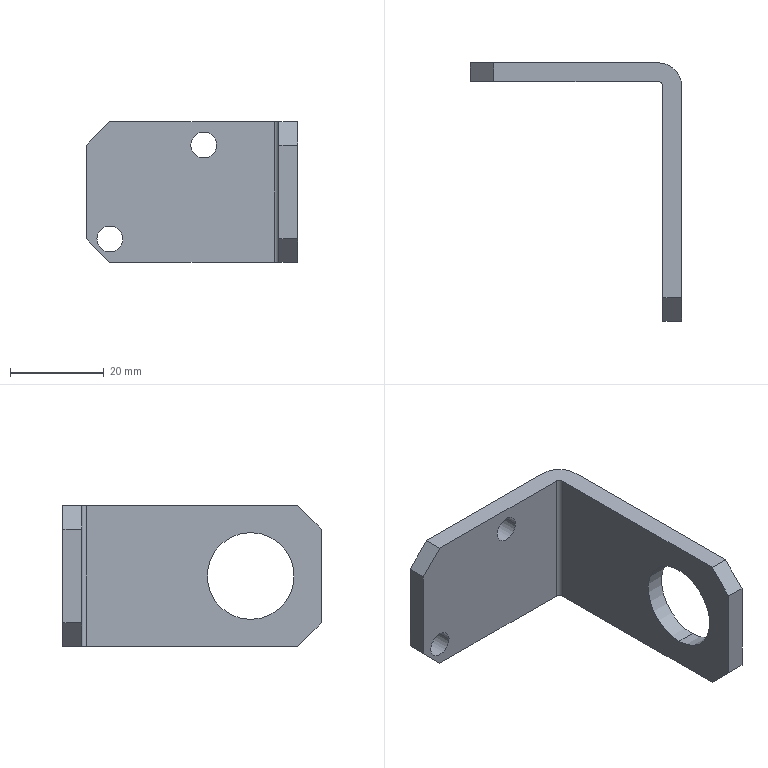Part | SolidWorks | features ICE 2, Chamfer 1, Extrusion 1 | 1 solid | 20 faces | box 45 x 55 x 30 mm | volume 9900 mm3 | plane 12 | cylinder 8 | commonest cylinder face diameters 5.5 x4 18.5 x2 2 x1 10 x1
STEP:
#1=CARTESIAN_POINT('',(7.75,-4.,5.));
#2=VERTEX_POINT('',#1);
#3=CARTESIAN_POINT('',(2.25,-4.,5.));
#4=VERTEX_POINT('',#3);
#5=CARTESIAN_POINT('',(5.,-4.,5.));
#6=DIRECTION('',(0.,1.,0.));
#7=DIRECTION('',(0.,0.,1.));
#8=AXIS2_PLACEMENT_3D('',#5,#6,#7);
#9=CIRCLE('',#8,2.75);
#10=EDGE_CURVE('',#2,#4,#9,.T.);
#11=ORIENTED_EDGE('',*,*,#10,.F.);
#12=CARTESIAN_POINT('',(7.75,0.,5.));
#13=VERTEX_POINT('',#12);
#14=CARTESIAN_POINT('',(7.75,-30.,5.));
#15=DIRECTION('',(0.,1.,0.));
#16=VECTOR('',#15,1000.);
#17=LINE('',#14,#16);
#18=EDGE_CURVE('',#2,#13,#17,.T.);
#19=ORIENTED_EDGE('',*,*,#18,.T.);
#20=CARTESIAN_POINT('',(2.25,0.,5.));
#21=VERTEX_POINT('',#20);
#22=CARTESIAN_POINT('',(5.,0.,5.));
#23=DIRECTION('',(0.,1.,0.));
#24=DIRECTION('',(-1.,0.,0.));
#25=AXIS2_PLACEMENT_3D('',#22,#23,#24);
#26=CIRCLE('',#25,2.75);
#27=EDGE_CURVE('',#13,#21,#26,.T.);
#28=ORIENTED_EDGE('',*,*,#27,.T.);
#29=CARTESIAN_POINT('',(2.25,-30.,5.));
#30=DIRECTION('',(0.,1.,0.));
#31=VECTOR('',#30,1000.);
#32=LINE('',#29,#31);
#33=EDGE_CURVE('',#4,#21,#32,.T.);
#34=ORIENTED_EDGE('',*,*,#33,.F.);
#35=EDGE_LOOP('',(#11,#19,#28,#34));
#36=FACE_OUTER_BOUND('',#35,.T.);
#37=CARTESIAN_POINT('',(5.,-30.,5.));
#38=DIRECTION('',(0.,1.,0.));
#39=DIRECTION('',(-1.,0.,0.));
#40=AXIS2_PLACEMENT_3D('',#37,#38,#39);
#41=CYLINDRICAL_SURFACE('',#40,2.75);
#42=ADVANCED_FACE('',(#36),#41,.F.);
#43=CARTESIAN_POINT('',(27.75,-4.,25.));
#44=VERTEX_POINT('',#43);
#45=CARTESIAN_POINT('',(22.25,-4.,25.));
#46=VERTEX_POINT('',#45);
#47=CARTESIAN_POINT('',(25.,-4.,25.));
#48=DIRECTION('',(0.,1.,0.));
#49=DIRECTION('',(0.,0.,1.));
#50=AXIS2_PLACEMENT_3D('',#47,#48,#49);
#51=CIRCLE('',#50,2.75);
#52=EDGE_CURVE('',#44,#46,#51,.T.);
#53=ORIENTED_EDGE('',*,*,#52,.F.);
#54=CARTESIAN_POINT('',(27.75,0.,25.));
#55=VERTEX_POINT('',#54);
#56=CARTESIAN_POINT('',(27.75,-30.,25.));
#57=DIRECTION('',(0.,1.,0.));
#58=VECTOR('',#57,1000.);
#59=LINE('',#56,#58);
#60=EDGE_CURVE('',#44,#55,#59,.T.);
#61=ORIENTED_EDGE('',*,*,#60,.T.);
#62=CARTESIAN_POINT('',(22.25,0.,25.));
#63=VERTEX_POINT('',#62);
#64=CARTESIAN_POINT('',(25.,0.,25.));
#65=DIRECTION('',(0.,1.,0.));
#66=DIRECTION('',(-1.,0.,0.));
#67=AXIS2_PLACEMENT_3D('',#64,#65,#66);
#68=CIRCLE('',#67,2.75);
#69=EDGE_CURVE('',#55,#63,#68,.T.);
#70=ORIENTED_EDGE('',*,*,#69,.T.);
#71=CARTESIAN_POINT('',(22.25,-30.,25.));
#72=DIRECTION('',(0.,1.,0.));
#73=VECTOR('',#72,1000.);
#74=LINE('',#71,#73);
#75=EDGE_CURVE('',#46,#63,#74,.T.);
#76=ORIENTED_EDGE('',*,*,#75,.F.);
#77=EDGE_LOOP('',(#53,#61,#70,#76));
#78=FACE_OUTER_BOUND('',#77,.T.);
#79=CARTESIAN_POINT('',(25.,-30.,25.));
#80=DIRECTION('',(0.,1.,0.));
#81=DIRECTION('',(-1.,0.,0.));
#82=AXIS2_PLACEMENT_3D('',#79,#80,#81);
#83=CYLINDRICAL_SURFACE('',#82,2.75);
#84=ADVANCED_FACE('',(#78),#83,.F.);
#85=CARTESIAN_POINT('',(41.,-40.,24.25));
#86=VERTEX_POINT('',#85);
#87=CARTESIAN_POINT('',(41.,-40.,5.75));
#88=VERTEX_POINT('',#87);
#89=CARTESIAN_POINT('',(41.,-40.,15.));
#90=DIRECTION('',(1.,0.,0.));
#91=DIRECTION('',(0.,1.,0.));
#92=AXIS2_PLACEMENT_3D('',#89,#90,#91);
#93=CIRCLE('',#92,9.25);
#94=EDGE_CURVE('',#86,#88,#93,.T.);
#95=ORIENTED_EDGE('',*,*,#94,.F.);
#96=CARTESIAN_POINT('',(45.,-40.,24.25));
#97=VERTEX_POINT('',#96);
#98=CARTESIAN_POINT('',(15.,-40.,24.25));
#99=DIRECTION('',(1.,0.,0.));
#100=VECTOR('',#99,1000.);
#101=LINE('',#98,#100);
#102=EDGE_CURVE('',#86,#97,#101,.T.);
#103=ORIENTED_EDGE('',*,*,#102,.T.);
#104=CARTESIAN_POINT('',(45.,-40.,5.75));
#105=VERTEX_POINT('',#104);
#106=CARTESIAN_POINT('',(45.,-40.,15.));
#107=DIRECTION('',(1.,0.,0.));
#108=DIRECTION('',(0.,0.,-1.));
#109=AXIS2_PLACEMENT_3D('',#106,#107,#108);
#110=CIRCLE('',#109,9.25);
#111=EDGE_CURVE('',#97,#105,#110,.T.);
#112=ORIENTED_EDGE('',*,*,#111,.T.);
#113=CARTESIAN_POINT('',(15.,-40.,5.75));
#114=DIRECTION('',(1.,0.,0.));
#115=VECTOR('',#114,1000.);
#116=LINE('',#113,#115);
#117=EDGE_CURVE('',#88,#105,#116,.T.);
#118=ORIENTED_EDGE('',*,*,#117,.F.);
#119=EDGE_LOOP('',(#95,#103,#112,#118));
#120=FACE_OUTER_BOUND('',#119,.T.);
#121=CARTESIAN_POINT('',(15.,-40.,15.));
#122=DIRECTION('',(1.,0.,0.));
#123=DIRECTION('',(0.,0.,-1.));
#124=AXIS2_PLACEMENT_3D('',#121,#122,#123);
#125=CYLINDRICAL_SURFACE('',#124,9.25);
#126=ADVANCED_FACE('',(#120),#125,.F.);
#127=CARTESIAN_POINT('',(45.,-40.,15.));
#128=DIRECTION('',(1.,0.,0.));
#129=DIRECTION('',(0.,0.,-1.));
#130=AXIS2_PLACEMENT_3D('',#127,#128,#129);
#131=CIRCLE('',#130,9.25);
#132=EDGE_CURVE('',#105,#97,#131,.T.);
#133=ORIENTED_EDGE('',*,*,#132,.F.);
#134=ORIENTED_EDGE('',*,*,#111,.F.);
#135=EDGE_LOOP('',(#133,#134));
#136=FACE_BOUND('',#135,.T.);
#137=CARTESIAN_POINT('',(45.,-55.,25.));
#138=VERTEX_POINT('',#137);
#139=CARTESIAN_POINT('',(45.,-55.,5.));
#140=VERTEX_POINT('',#139);
#141=CARTESIAN_POINT('',(45.,-55.,30.));
#142=DIRECTION('',(0.,0.,-1.));
#143=VECTOR('',#142,1000.);
#144=LINE('',#141,#143);
#145=EDGE_CURVE('',#138,#140,#144,.T.);
#146=ORIENTED_EDGE('',*,*,#145,.T.);
#147=CARTESIAN_POINT('',(45.,-50.,0.));
#148=VERTEX_POINT('',#147);
#149=CARTESIAN_POINT('',(45.,-42.5,-7.5));
#150=DIRECTION('',(0.,0.7071,-0.7071));
#151=VECTOR('',#150,1000.);
#152=LINE('',#149,#151);
#153=EDGE_CURVE('',#140,#148,#152,.T.);
#154=ORIENTED_EDGE('',*,*,#153,.T.);
#155=CARTESIAN_POINT('',(45.,-5.,0.));
#156=VERTEX_POINT('',#155);
#157=CARTESIAN_POINT('',(45.,-5.,0.));
#158=DIRECTION('',(0.,-1.,0.));
#159=VECTOR('',#158,1000.);
#160=LINE('',#157,#159);
#161=EDGE_CURVE('',#156,#148,#160,.T.);
#162=ORIENTED_EDGE('',*,*,#161,.F.);
#163=CARTESIAN_POINT('',(45.,-5.,30.));
#164=VERTEX_POINT('',#163);
#165=CARTESIAN_POINT('',(45.,-5.,30.));
#166=DIRECTION('',(0.,0.,-1.));
#167=VECTOR('',#166,1000.);
#168=LINE('',#165,#167);
#169=EDGE_CURVE('',#164,#156,#168,.T.);
#170=ORIENTED_EDGE('',*,*,#169,.F.);
#171=CARTESIAN_POINT('',(45.,-50.,30.));
#172=VERTEX_POINT('',#171);
#173=CARTESIAN_POINT('',(45.,-5.,30.));
#174=DIRECTION('',(0.,-1.,0.));
#175=VECTOR('',#174,1000.);
#176=LINE('',#173,#175);
#177=EDGE_CURVE('',#164,#172,#176,.T.);
#178=ORIENTED_EDGE('',*,*,#177,.T.);
#179=CARTESIAN_POINT('',(45.,-27.5,52.5));
#180=DIRECTION('',(0.,-0.7071,-0.7071));
#181=VECTOR('',#180,1000.);
#182=LINE('',#179,#181);
#183=EDGE_CURVE('',#172,#138,#182,.T.);
#184=ORIENTED_EDGE('',*,*,#183,.T.);
#185=EDGE_LOOP('',(#146,#154,#162,#170,#178,#184));
#186=FACE_OUTER_BOUND('',#185,.T.);
#187=CARTESIAN_POINT('',(45.,-5.,30.));
#188=DIRECTION('',(1.,0.,0.));
#189=DIRECTION('',(0.,0.,-1.));
#190=AXIS2_PLACEMENT_3D('',#187,#188,#189);
#191=PLANE('',#190);
#192=ADVANCED_FACE('',(#136,#186),#191,.T.);
#193=CARTESIAN_POINT('',(40.,0.,0.));
#194=VERTEX_POINT('',#193);
#195=CARTESIAN_POINT('',(40.,-5.,0.));
#196=DIRECTION('',(0.,0.,-1.));
#197=DIRECTION('',(-1.,0.,0.));
#198=AXIS2_PLACEMENT_3D('',#195,#196,#197);
#199=CIRCLE('',#198,5.);
#200=EDGE_CURVE('',#194,#156,#199,.T.);
#201=ORIENTED_EDGE('',*,*,#200,.F.);
#202=CARTESIAN_POINT('',(40.,0.,30.));
#203=VERTEX_POINT('',#202);
#204=CARTESIAN_POINT('',(40.,0.,30.));
#205=DIRECTION('',(0.,0.,-1.));
#206=VECTOR('',#205,1000.);
#207=LINE('',#204,#206);
#208=EDGE_CURVE('',#203,#194,#207,.T.);
#209=ORIENTED_EDGE('',*,*,#208,.F.);
#210=CARTESIAN_POINT('',(40.,-5.,30.));
#211=DIRECTION('',(0.,0.,-1.));
#212=DIRECTION('',(-1.,0.,0.));
#213=AXIS2_PLACEMENT_3D('',#210,#211,#212);
#214=CIRCLE('',#213,5.);
#215=EDGE_CURVE('',#203,#164,#214,.T.);
#216=ORIENTED_EDGE('',*,*,#215,.T.);
#217=ORIENTED_EDGE('',*,*,#169,.T.);
#218=EDGE_LOOP('',(#201,#209,#216,#217));
#219=FACE_OUTER_BOUND('',#218,.T.);
#220=CARTESIAN_POINT('',(40.,-5.,30.));
#221=DIRECTION('',(0.,0.,-1.));
#222=DIRECTION('',(-1.,0.,0.));
#223=AXIS2_PLACEMENT_3D('',#220,#221,#222);
#224=CYLINDRICAL_SURFACE('',#223,5.);
#225=ADVANCED_FACE('',(#219),#224,.T.);
#226=CARTESIAN_POINT('',(5.,0.,5.));
#227=DIRECTION('',(0.,1.,0.));
#228=DIRECTION('',(-1.,0.,0.));
#229=AXIS2_PLACEMENT_3D('',#226,#227,#228);
#230=CIRCLE('',#229,2.75);
#231=EDGE_CURVE('',#21,#13,#230,.T.);
#232=ORIENTED_EDGE('',*,*,#231,.F.);
#233=ORIENTED_EDGE('',*,*,#27,.F.);
#234=EDGE_LOOP('',(#232,#233));
#235=FACE_BOUND('',#234,.T.);
#236=CARTESIAN_POINT('',(25.,0.,25.));
#237=DIRECTION('',(0.,1.,0.));
#238=DIRECTION('',(-1.,0.,0.));
#239=AXIS2_PLACEMENT_3D('',#236,#237,#238);
#240=CIRCLE('',#239,2.75);
#241=EDGE_CURVE('',#63,#55,#240,.T.);
#242=ORIENTED_EDGE('',*,*,#241,.F.);
#243=ORIENTED_EDGE('',*,*,#69,.F.);
#244=EDGE_LOOP('',(#242,#243));
#245=FACE_BOUND('',#244,.T.);
#246=CARTESIAN_POINT('',(5.,0.,0.));
#247=VERTEX_POINT('',#246);
#248=CARTESIAN_POINT('',(0.,0.,0.));
#249=DIRECTION('',(1.,0.,0.));
#250=VECTOR('',#249,1000.);
#251=LINE('',#248,#250);
#252=EDGE_CURVE('',#247,#194,#251,.T.);
#253=ORIENTED_EDGE('',*,*,#252,.F.);
#254=CARTESIAN_POINT('',(0.,0.,5.));
#255=VERTEX_POINT('',#254);
#256=CARTESIAN_POINT('',(-12.5,0.,17.5));
#257=DIRECTION('',(-0.7071,0.,0.7071));
#258=VECTOR('',#257,1000.);
#259=LINE('',#256,#258);
#260=EDGE_CURVE('',#247,#255,#259,.T.);
#261=ORIENTED_EDGE('',*,*,#260,.T.);
#262=CARTESIAN_POINT('',(0.,0.,25.));
#263=VERTEX_POINT('',#262);
#264=CARTESIAN_POINT('',(0.,0.,30.));
#265=DIRECTION('',(0.,0.,-1.));
#266=VECTOR('',#265,1000.);
#267=LINE('',#264,#266);
#268=EDGE_CURVE('',#263,#255,#267,.T.);
#269=ORIENTED_EDGE('',*,*,#268,.F.);
#270=CARTESIAN_POINT('',(5.,0.,30.));
#271=VERTEX_POINT('',#270);
#272=CARTESIAN_POINT('',(2.5,0.,27.5));
#273=DIRECTION('',(0.7071,0.,0.7071));
#274=VECTOR('',#273,1000.);
#275=LINE('',#272,#274);
#276=EDGE_CURVE('',#263,#271,#275,.T.);
#277=ORIENTED_EDGE('',*,*,#276,.T.);
#278=CARTESIAN_POINT('',(0.,0.,30.));
#279=DIRECTION('',(1.,0.,0.));
#280=VECTOR('',#279,1000.);
#281=LINE('',#278,#280);
#282=EDGE_CURVE('',#271,#203,#281,.T.);
#283=ORIENTED_EDGE('',*,*,#282,.T.);
#284=ORIENTED_EDGE('',*,*,#208,.T.);
#285=EDGE_LOOP('',(#253,#261,#269,#277,#283,#284));
#286=FACE_OUTER_BOUND('',#285,.T.);
#287=CARTESIAN_POINT('',(0.,0.,30.));
#288=DIRECTION('',(0.,1.,0.));
#289=DIRECTION('',(-1.,0.,0.));
#290=AXIS2_PLACEMENT_3D('',#287,#288,#289);
#291=PLANE('',#290);
#292=ADVANCED_FACE('',(#235,#245,#286),#291,.T.);
#293=ORIENTED_EDGE('',*,*,#268,.T.);
#294=CARTESIAN_POINT('',(0.,-4.,5.));
#295=VERTEX_POINT('',#294);
#296=CARTESIAN_POINT('',(0.,-4.,5.));
#297=DIRECTION('',(0.,-1.,0.));
#298=VECTOR('',#297,1000.);
#299=LINE('',#296,#298);
#300=EDGE_CURVE('',#255,#295,#299,.T.);
#301=ORIENTED_EDGE('',*,*,#300,.T.);
#302=CARTESIAN_POINT('',(0.,-4.,25.));
#303=VERTEX_POINT('',#302);
#304=CARTESIAN_POINT('',(0.,-4.,30.));
#305=DIRECTION('',(0.,0.,-1.));
#306=VECTOR('',#305,1000.);
#307=LINE('',#304,#306);
#308=EDGE_CURVE('',#303,#295,#307,.T.);
#309=ORIENTED_EDGE('',*,*,#308,.F.);
#310=CARTESIAN_POINT('',(0.,0.,25.));
#311=DIRECTION('',(0.,1.,0.));
#312=VECTOR('',#311,1000.);
#313=LINE('',#310,#312);
#314=EDGE_CURVE('',#303,#263,#313,.T.);
#315=ORIENTED_EDGE('',*,*,#314,.T.);
#316=EDGE_LOOP('',(#293,#301,#309,#315));
#317=FACE_OUTER_BOUND('',#316,.T.);
#318=CARTESIAN_POINT('',(0.,0.,30.));
#319=DIRECTION('',(1.,0.,0.));
#320=DIRECTION('',(0.,0.,-1.));
#321=AXIS2_PLACEMENT_3D('',#318,#319,#320);
#322=PLANE('',#321);
#323=ADVANCED_FACE('',(#317),#322,.F.);
#324=CARTESIAN_POINT('',(5.,-4.,5.));
#325=DIRECTION('',(0.,1.,0.));
#326=DIRECTION('',(0.,0.,1.));
#327=AXIS2_PLACEMENT_3D('',#324,#325,#326);
#328=CIRCLE('',#327,2.75);
#329=EDGE_CURVE('',#4,#2,#328,.T.);
#330=ORIENTED_EDGE('',*,*,#329,.T.);
#331=ORIENTED_EDGE('',*,*,#10,.T.);
#332=EDGE_LOOP('',(#330,#331));
#333=FACE_BOUND('',#332,.T.);
#334=CARTESIAN_POINT('',(25.,-4.,25.));
#335=DIRECTION('',(0.,1.,0.));
#336=DIRECTION('',(0.,0.,1.));
#337=AXIS2_PLACEMENT_3D('',#334,#335,#336);
#338=CIRCLE('',#337,2.75);
#339=EDGE_CURVE('',#46,#44,#338,.T.);
#340=ORIENTED_EDGE('',*,*,#339,.T.);
#341=ORIENTED_EDGE('',*,*,#52,.T.);
#342=EDGE_LOOP('',(#340,#341));
#343=FACE_BOUND('',#342,.T.);
#344=ORIENTED_EDGE('',*,*,#308,.T.);
#345=CARTESIAN_POINT('',(5.,-4.,0.));
#346=VERTEX_POINT('',#345);
#347=CARTESIAN_POINT('',(0.,-4.,5.));
#348=DIRECTION('',(0.7071,0.,-0.7071));
#349=VECTOR('',#348,1000.);
#350=LINE('',#347,#349);
#351=EDGE_CURVE('',#295,#346,#350,.T.);
#352=ORIENTED_EDGE('',*,*,#351,.T.);
#353=CARTESIAN_POINT('',(40.,-4.,0.));
#354=VERTEX_POINT('',#353);
#355=CARTESIAN_POINT('',(0.,-4.,0.));
#356=DIRECTION('',(1.,0.,0.));
#357=VECTOR('',#356,1000.);
#358=LINE('',#355,#357);
#359=EDGE_CURVE('',#346,#354,#358,.T.);
#360=ORIENTED_EDGE('',*,*,#359,.T.);
#361=CARTESIAN_POINT('',(40.,-4.,30.));
#362=VERTEX_POINT('',#361);
#363=CARTESIAN_POINT('',(40.,-4.,30.));
#364=DIRECTION('',(0.,0.,-1.));
#365=VECTOR('',#364,1000.);
#366=LINE('',#363,#365);
#367=EDGE_CURVE('',#362,#354,#366,.T.);
#368=ORIENTED_EDGE('',*,*,#367,.F.);
#369=CARTESIAN_POINT('',(5.,-4.,30.));
#370=VERTEX_POINT('',#369);
#371=CARTESIAN_POINT('',(0.,-4.,30.));
#372=DIRECTION('',(1.,0.,0.));
#373=VECTOR('',#372,1000.);
#374=LINE('',#371,#373);
#375=EDGE_CURVE('',#370,#362,#374,.T.);
#376=ORIENTED_EDGE('',*,*,#375,.F.);
#377=CARTESIAN_POINT('',(5.,-4.,30.));
#378=DIRECTION('',(-0.7071,0.,-0.7071));
#379=VECTOR('',#378,1000.);
#380=LINE('',#377,#379);
#381=EDGE_CURVE('',#370,#303,#380,.T.);
#382=ORIENTED_EDGE('',*,*,#381,.T.);
#383=EDGE_LOOP('',(#344,#352,#360,#368,#376,#382));
#384=FACE_OUTER_BOUND('',#383,.T.);
#385=CARTESIAN_POINT('',(0.,-4.,30.));
#386=DIRECTION('',(0.,1.,0.));
#387=DIRECTION('',(0.,0.,1.));
#388=AXIS2_PLACEMENT_3D('',#385,#386,#387);
#389=PLANE('',#388);
#390=ADVANCED_FACE('',(#333,#343,#384),#389,.F.);
#391=CARTESIAN_POINT('',(41.,-5.,0.));
#392=VERTEX_POINT('',#391);
#393=CARTESIAN_POINT('',(40.,-5.,0.));
#394=DIRECTION('',(0.,0.,-1.));
#395=DIRECTION('',(-1.,0.,0.));
#396=AXIS2_PLACEMENT_3D('',#393,#394,#395);
#397=CIRCLE('',#396,1.);
#398=EDGE_CURVE('',#354,#392,#397,.T.);
#399=ORIENTED_EDGE('',*,*,#398,.T.);
#400=CARTESIAN_POINT('',(41.,-5.,30.));
#401=VERTEX_POINT('',#400);
#402=CARTESIAN_POINT('',(41.,-5.,30.));
#403=DIRECTION('',(0.,0.,-1.));
#404=VECTOR('',#403,1000.);
#405=LINE('',#402,#404);
#406=EDGE_CURVE('',#401,#392,#405,.T.);
#407=ORIENTED_EDGE('',*,*,#406,.F.);
#408=CARTESIAN_POINT('',(40.,-5.,30.));
#409=DIRECTION('',(0.,0.,-1.));
#410=DIRECTION('',(-1.,0.,0.));
#411=AXIS2_PLACEMENT_3D('',#408,#409,#410);
#412=CIRCLE('',#411,1.);
#413=EDGE_CURVE('',#362,#401,#412,.T.);
#414=ORIENTED_EDGE('',*,*,#413,.F.);
#415=ORIENTED_EDGE('',*,*,#367,.T.);
#416=EDGE_LOOP('',(#399,#407,#414,#415));
#417=FACE_OUTER_BOUND('',#416,.T.);
#418=CARTESIAN_POINT('',(40.,-5.,30.));
#419=DIRECTION('',(0.,0.,-1.));
#420=DIRECTION('',(-1.,0.,0.));
#421=AXIS2_PLACEMENT_3D('',#418,#419,#420);
#422=CYLINDRICAL_SURFACE('',#421,1.);
#423=ADVANCED_FACE('',(#417),#422,.F.);
#424=CARTESIAN_POINT('',(41.,-40.,15.));
#425=DIRECTION('',(1.,0.,0.));
#426=DIRECTION('',(0.,1.,0.));
#427=AXIS2_PLACEMENT_3D('',#424,#425,#426);
#428=CIRCLE('',#427,9.25);
#429=EDGE_CURVE('',#88,#86,#428,.T.);
#430=ORIENTED_EDGE('',*,*,#429,.T.);
#431=ORIENTED_EDGE('',*,*,#94,.T.);
#432=EDGE_LOOP('',(#430,#431));
#433=FACE_BOUND('',#432,.T.);
#434=CARTESIAN_POINT('',(41.,-50.,0.));
#435=VERTEX_POINT('',#434);
#436=CARTESIAN_POINT('',(41.,-5.,0.));
#437=DIRECTION('',(0.,-1.,0.));
#438=VECTOR('',#437,1000.);
#439=LINE('',#436,#438);
#440=EDGE_CURVE('',#392,#435,#439,.T.);
#441=ORIENTED_EDGE('',*,*,#440,.T.);
#442=CARTESIAN_POINT('',(41.,-55.,5.));
#443=VERTEX_POINT('',#442);
#444=CARTESIAN_POINT('',(41.,-50.,0.));
#445=DIRECTION('',(0.,-0.7071,0.7071));
#446=VECTOR('',#445,1000.);
#447=LINE('',#444,#446);
#448=EDGE_CURVE('',#435,#443,#447,.T.);
#449=ORIENTED_EDGE('',*,*,#448,.T.);
#450=CARTESIAN_POINT('',(41.,-55.,25.));
#451=VERTEX_POINT('',#450);
#452=CARTESIAN_POINT('',(41.,-55.,30.));
#453=DIRECTION('',(0.,0.,-1.));
#454=VECTOR('',#453,1000.);
#455=LINE('',#452,#454);
#456=EDGE_CURVE('',#451,#443,#455,.T.);
#457=ORIENTED_EDGE('',*,*,#456,.F.);
#458=CARTESIAN_POINT('',(41.,-50.,30.));
#459=VERTEX_POINT('',#458);
#460=CARTESIAN_POINT('',(41.,-55.,25.));
#461=DIRECTION('',(0.,0.7071,0.7071));
#462=VECTOR('',#461,1000.);
#463=LINE('',#460,#462);
#464=EDGE_CURVE('',#451,#459,#463,.T.);
#465=ORIENTED_EDGE('',*,*,#464,.T.);
#466=CARTESIAN_POINT('',(41.,-5.,30.));
#467=DIRECTION('',(0.,-1.,0.));
#468=VECTOR('',#467,1000.);
#469=LINE('',#466,#468);
#470=EDGE_CURVE('',#401,#459,#469,.T.);
#471=ORIENTED_EDGE('',*,*,#470,.F.);
#472=ORIENTED_EDGE('',*,*,#406,.T.);
#473=EDGE_LOOP('',(#441,#449,#457,#465,#471,#472));
#474=FACE_OUTER_BOUND('',#473,.T.);
#475=CARTESIAN_POINT('',(41.,-5.,30.));
#476=DIRECTION('',(1.,0.,0.));
#477=DIRECTION('',(0.,1.,0.));
#478=AXIS2_PLACEMENT_3D('',#475,#476,#477);
#479=PLANE('',#478);
#480=ADVANCED_FACE('',(#433,#474),#479,.F.);
#481=ORIENTED_EDGE('',*,*,#456,.T.);
#482=CARTESIAN_POINT('',(45.,-55.,5.));
#483=DIRECTION('',(1.,0.,0.));
#484=VECTOR('',#483,1000.);
#485=LINE('',#482,#484);
#486=EDGE_CURVE('',#443,#140,#485,.T.);
#487=ORIENTED_EDGE('',*,*,#486,.T.);
#488=ORIENTED_EDGE('',*,*,#145,.F.);
#489=CARTESIAN_POINT('',(41.,-55.,25.));
#490=DIRECTION('',(-1.,0.,0.));
#491=VECTOR('',#490,1000.);
#492=LINE('',#489,#491);
#493=EDGE_CURVE('',#138,#451,#492,.T.);
#494=ORIENTED_EDGE('',*,*,#493,.T.);
#495=EDGE_LOOP('',(#481,#487,#488,#494));
#496=FACE_OUTER_BOUND('',#495,.T.);
#497=CARTESIAN_POINT('',(45.,-55.,30.));
#498=DIRECTION('',(0.,-1.,0.));
#499=DIRECTION('',(0.,0.,-1.));
#500=AXIS2_PLACEMENT_3D('',#497,#498,#499);
#501=PLANE('',#500);
#502=ADVANCED_FACE('',(#496),#501,.T.);
#503=ORIENTED_EDGE('',*,*,#470,.T.);
#504=CARTESIAN_POINT('',(45.,-50.,30.));
#505=DIRECTION('',(1.,0.,0.));
#506=VECTOR('',#505,1000.);
#507=LINE('',#504,#506);
#508=EDGE_CURVE('',#459,#172,#507,.T.);
#509=ORIENTED_EDGE('',*,*,#508,.T.);
#510=ORIENTED_EDGE('',*,*,#177,.F.);
#511=ORIENTED_EDGE('',*,*,#215,.F.);
#512=ORIENTED_EDGE('',*,*,#282,.F.);
#513=CARTESIAN_POINT('',(5.,-5.,30.));
#514=DIRECTION('',(0.,-1.,0.));
#515=VECTOR('',#514,1000.);
#516=LINE('',#513,#515);
#517=EDGE_CURVE('',#271,#370,#516,.T.);
#518=ORIENTED_EDGE('',*,*,#517,.T.);
#519=ORIENTED_EDGE('',*,*,#375,.T.);
#520=ORIENTED_EDGE('',*,*,#413,.T.);
#521=EDGE_LOOP('',(#503,#509,#510,#511,#512,#518,#519,#520));
#522=FACE_OUTER_BOUND('',#521,.T.);
#523=CARTESIAN_POINT('',(40.,-5.,30.));
#524=DIRECTION('',(0.,0.,-1.));
#525=DIRECTION('',(-1.,0.,0.));
#526=AXIS2_PLACEMENT_3D('',#523,#524,#525);
#527=PLANE('',#526);
#528=ADVANCED_FACE('',(#522),#527,.F.);
#529=ORIENTED_EDGE('',*,*,#161,.T.);
#530=CARTESIAN_POINT('',(40.,-50.,0.));
#531=DIRECTION('',(-1.,0.,0.));
#532=VECTOR('',#531,1000.);
#533=LINE('',#530,#532);
#534=EDGE_CURVE('',#148,#435,#533,.T.);
#535=ORIENTED_EDGE('',*,*,#534,.T.);
#536=ORIENTED_EDGE('',*,*,#440,.F.);
#537=ORIENTED_EDGE('',*,*,#398,.F.);
#538=ORIENTED_EDGE('',*,*,#359,.F.);
#539=CARTESIAN_POINT('',(5.,0.,0.));
#540=DIRECTION('',(0.,1.,0.));
#541=VECTOR('',#540,1000.);
#542=LINE('',#539,#541);
#543=EDGE_CURVE('',#346,#247,#542,.T.);
#544=ORIENTED_EDGE('',*,*,#543,.T.);
#545=ORIENTED_EDGE('',*,*,#252,.T.);
#546=ORIENTED_EDGE('',*,*,#200,.T.);
#547=EDGE_LOOP('',(#529,#535,#536,#537,#538,#544,#545,#546));
#548=FACE_OUTER_BOUND('',#547,.T.);
#549=CARTESIAN_POINT('',(40.,-5.,0.));
#550=DIRECTION('',(0.,0.,-1.));
#551=DIRECTION('',(-1.,0.,0.));
#552=AXIS2_PLACEMENT_3D('',#549,#550,#551);
#553=PLANE('',#552);
#554=ADVANCED_FACE('',(#548),#553,.T.);
#555=ORIENTED_EDGE('',*,*,#102,.F.);
#556=ORIENTED_EDGE('',*,*,#429,.F.);
#557=ORIENTED_EDGE('',*,*,#117,.T.);
#558=ORIENTED_EDGE('',*,*,#132,.T.);
#559=EDGE_LOOP('',(#555,#556,#557,#558));
#560=FACE_OUTER_BOUND('',#559,.T.);
#561=CARTESIAN_POINT('',(15.,-40.,15.));
#562=DIRECTION('',(1.,0.,0.));
#563=DIRECTION('',(0.,0.,-1.));
#564=AXIS2_PLACEMENT_3D('',#561,#562,#563);
#565=CYLINDRICAL_SURFACE('',#564,9.25);
#566=ADVANCED_FACE('',(#560),#565,.F.);
#567=ORIENTED_EDGE('',*,*,#60,.F.);
#568=ORIENTED_EDGE('',*,*,#339,.F.);
#569=ORIENTED_EDGE('',*,*,#75,.T.);
#570=ORIENTED_EDGE('',*,*,#241,.T.);
#571=EDGE_LOOP('',(#567,#568,#569,#570));
#572=FACE_OUTER_BOUND('',#571,.T.);
#573=CARTESIAN_POINT('',(25.,-30.,25.));
#574=DIRECTION('',(0.,1.,0.));
#575=DIRECTION('',(-1.,0.,0.));
#576=AXIS2_PLACEMENT_3D('',#573,#574,#575);
#577=CYLINDRICAL_SURFACE('',#576,2.75);
#578=ADVANCED_FACE('',(#572),#577,.F.);
#579=ORIENTED_EDGE('',*,*,#18,.F.);
#580=ORIENTED_EDGE('',*,*,#329,.F.);
#581=ORIENTED_EDGE('',*,*,#33,.T.);
#582=ORIENTED_EDGE('',*,*,#231,.T.);
#583=EDGE_LOOP('',(#579,#580,#581,#582));
#584=FACE_OUTER_BOUND('',#583,.T.);
#585=CARTESIAN_POINT('',(5.,-30.,5.));
#586=DIRECTION('',(0.,1.,0.));
#587=DIRECTION('',(-1.,0.,0.));
#588=AXIS2_PLACEMENT_3D('',#585,#586,#587);
#589=CYLINDRICAL_SURFACE('',#588,2.75);
#590=ADVANCED_FACE('',(#584),#589,.F.);
#591=ORIENTED_EDGE('',*,*,#153,.F.);
#592=ORIENTED_EDGE('',*,*,#486,.F.);
#593=ORIENTED_EDGE('',*,*,#448,.F.);
#594=ORIENTED_EDGE('',*,*,#534,.F.);
#595=EDGE_LOOP('',(#591,#592,#593,#594));
#596=FACE_OUTER_BOUND('',#595,.T.);
#597=CARTESIAN_POINT('',(40.,-50.,0.));
#598=DIRECTION('',(0.,0.7071,0.7071));
#599=DIRECTION('',(-1.,0.,0.));
#600=AXIS2_PLACEMENT_3D('',#597,#598,#599);
#601=PLANE('',#600);
#602=ADVANCED_FACE('',(#596),#601,.F.);
#603=ORIENTED_EDGE('',*,*,#183,.F.);
#604=ORIENTED_EDGE('',*,*,#508,.F.);
#605=ORIENTED_EDGE('',*,*,#464,.F.);
#606=ORIENTED_EDGE('',*,*,#493,.F.);
#607=EDGE_LOOP('',(#603,#604,#605,#606));
#608=FACE_OUTER_BOUND('',#607,.T.);
#609=CARTESIAN_POINT('',(45.,-55.,25.));
#610=DIRECTION('',(0.,-0.7071,0.7071));
#611=DIRECTION('',(1.,0.,0.));
#612=AXIS2_PLACEMENT_3D('',#609,#610,#611);
#613=PLANE('',#612);
#614=ADVANCED_FACE('',(#608),#613,.T.);
#615=ORIENTED_EDGE('',*,*,#260,.F.);
#616=ORIENTED_EDGE('',*,*,#543,.F.);
#617=ORIENTED_EDGE('',*,*,#351,.F.);
#618=ORIENTED_EDGE('',*,*,#300,.F.);
#619=EDGE_LOOP('',(#615,#616,#617,#618));
#620=FACE_OUTER_BOUND('',#619,.T.);
#621=CARTESIAN_POINT('',(0.,0.,5.));
#622=DIRECTION('',(-0.7071,0.,-0.7071));
#623=DIRECTION('',(0.,1.,0.));
#624=AXIS2_PLACEMENT_3D('',#621,#622,#623);
#625=PLANE('',#624);
#626=ADVANCED_FACE('',(#620),#625,.T.);
#627=ORIENTED_EDGE('',*,*,#276,.F.);
#628=ORIENTED_EDGE('',*,*,#314,.F.);
#629=ORIENTED_EDGE('',*,*,#381,.F.);
#630=ORIENTED_EDGE('',*,*,#517,.F.);
#631=EDGE_LOOP('',(#627,#628,#629,#630));
#632=FACE_OUTER_BOUND('',#631,.T.);
#633=CARTESIAN_POINT('',(5.,-5.,30.));
#634=DIRECTION('',(0.7071,0.,-0.7071));
#635=DIRECTION('',(0.,-1.,0.));
#636=AXIS2_PLACEMENT_3D('',#633,#634,#635);
#637=PLANE('',#636);
#638=ADVANCED_FACE('',(#632),#637,.F.);
#639=CLOSED_SHELL('',(#42,#84,#126,#192,#225,#292,#323,#390,#423,#480,#502,#528,#554,#566,#578,#590,#602,#614,#626,#638));
#640=MANIFOLD_SOLID_BREP('',#639);
#641=CARTESIAN_POINT('',(0.,0.,0.));
#642=DIRECTION('',(0.,0.,1.));
#643=DIRECTION('',(1.,0.,0.));
#644=AXIS2_PLACEMENT_3D('',#641,#642,#643);
#645=(LENGTH_UNIT()NAMED_UNIT(*)SI_UNIT(.MILLI.,.METRE.));
#646=UNCERTAINTY_MEASURE_WITH_UNIT(LENGTH_MEASURE(0.00001),#645,'','');
#647=(NAMED_UNIT(*)PLANE_ANGLE_UNIT()SI_UNIT($,.RADIAN.));
#648=(NAMED_UNIT(*)SI_UNIT($,.STERADIAN.)SOLID_ANGLE_UNIT());
#649=(GEOMETRIC_REPRESENTATION_CONTEXT(3)GLOBAL_UNCERTAINTY_ASSIGNED_CONTEXT((#646))GLOBAL_UNIT_ASSIGNED_CONTEXT((#645,#647,#648))REPRESENTATION_CONTEXT('',''));
#650=ADVANCED_BREP_SHAPE_REPRESENTATION('',(#640,#644),#649);